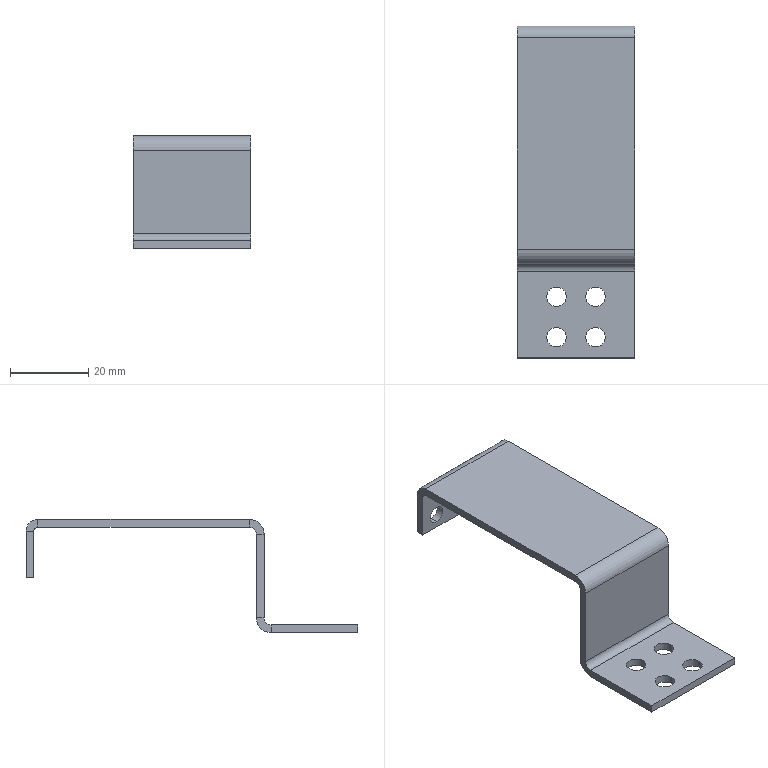Part | SolidWorks | features EdgeFlange 3, HoleWzd 2, FlatPattern 1, SMBaseFlange 1, SheetMetal 1 | 1 solid | 42 faces | box 30 x 85 x 29 mm | volume 7084 mm3 | plane 24 | cylinder 18 | commonest cylinder face diameters 5 x8 4.5 x4 3.6 x2 7.6 x2 2 x1 6 x1
STEP:
#1=CARTESIAN_POINT('',(-59.759,21.133,-13.25));
#2=VERTEX_POINT('',#1);
#3=CARTESIAN_POINT('',(-59.759,21.133,-8.75));
#4=VERTEX_POINT('',#3);
#5=CARTESIAN_POINT('',(-59.759,21.133,-11.));
#6=DIRECTION('',(0.,1.,0.));
#7=DIRECTION('',(0.,0.,1.));
#8=AXIS2_PLACEMENT_3D('',#5,#6,#7);
#9=CIRCLE('',#8,2.25);
#10=EDGE_CURVE('',#2,#4,#9,.T.);
#11=ORIENTED_EDGE('',*,*,#10,.T.);
#12=CARTESIAN_POINT('',(-59.759,19.133,-8.75));
#13=VERTEX_POINT('',#12);
#14=CARTESIAN_POINT('',(-59.759,19.133,-8.75));
#15=DIRECTION('',(0.,-1.,0.));
#16=VECTOR('',#15,1000.);
#17=LINE('',#14,#16);
#18=EDGE_CURVE('',#4,#13,#17,.T.);
#19=ORIENTED_EDGE('',*,*,#18,.T.);
#20=CARTESIAN_POINT('',(-59.759,19.133,-13.25));
#21=VERTEX_POINT('',#20);
#22=CARTESIAN_POINT('',(-59.759,19.133,-11.));
#23=DIRECTION('',(0.,-1.,0.));
#24=DIRECTION('',(0.,0.,-1.));
#25=AXIS2_PLACEMENT_3D('',#22,#23,#24);
#26=CIRCLE('',#25,2.25);
#27=EDGE_CURVE('',#13,#21,#26,.T.);
#28=ORIENTED_EDGE('',*,*,#27,.T.);
#29=CARTESIAN_POINT('',(-59.759,19.133,-13.25));
#30=DIRECTION('',(0.,-1.,0.));
#31=VECTOR('',#30,1000.);
#32=LINE('',#29,#31);
#33=EDGE_CURVE('',#2,#21,#32,.T.);
#34=ORIENTED_EDGE('',*,*,#33,.F.);
#35=EDGE_LOOP('',(#11,#19,#28,#34));
#36=FACE_OUTER_BOUND('',#35,.T.);
#37=CARTESIAN_POINT('',(-59.759,19.133,-11.));
#38=DIRECTION('',(0.,-1.,0.));
#39=DIRECTION('',(0.,0.,-1.));
#40=AXIS2_PLACEMENT_3D('',#37,#38,#39);
#41=CYLINDRICAL_SURFACE('',#40,2.25);
#42=ADVANCED_FACE('',(#36),#41,.F.);
#43=CARTESIAN_POINT('',(-39.759,21.133,-13.25));
#44=VERTEX_POINT('',#43);
#45=CARTESIAN_POINT('',(-39.759,21.133,-8.75));
#46=VERTEX_POINT('',#45);
#47=CARTESIAN_POINT('',(-39.759,21.133,-11.));
#48=DIRECTION('',(0.,1.,0.));
#49=DIRECTION('',(0.,0.,1.));
#50=AXIS2_PLACEMENT_3D('',#47,#48,#49);
#51=CIRCLE('',#50,2.25);
#52=EDGE_CURVE('',#44,#46,#51,.T.);
#53=ORIENTED_EDGE('',*,*,#52,.T.);
#54=CARTESIAN_POINT('',(-39.759,19.133,-8.75));
#55=VERTEX_POINT('',#54);
#56=CARTESIAN_POINT('',(-39.759,19.133,-8.75));
#57=DIRECTION('',(0.,-1.,0.));
#58=VECTOR('',#57,1000.);
#59=LINE('',#56,#58);
#60=EDGE_CURVE('',#46,#55,#59,.T.);
#61=ORIENTED_EDGE('',*,*,#60,.T.);
#62=CARTESIAN_POINT('',(-39.759,19.133,-13.25));
#63=VERTEX_POINT('',#62);
#64=CARTESIAN_POINT('',(-39.759,19.133,-11.));
#65=DIRECTION('',(0.,-1.,0.));
#66=DIRECTION('',(0.,0.,-1.));
#67=AXIS2_PLACEMENT_3D('',#64,#65,#66);
#68=CIRCLE('',#67,2.25);
#69=EDGE_CURVE('',#55,#63,#68,.T.);
#70=ORIENTED_EDGE('',*,*,#69,.T.);
#71=CARTESIAN_POINT('',(-39.759,19.133,-13.25));
#72=DIRECTION('',(0.,-1.,0.));
#73=VECTOR('',#72,1000.);
#74=LINE('',#71,#73);
#75=EDGE_CURVE('',#44,#63,#74,.T.);
#76=ORIENTED_EDGE('',*,*,#75,.F.);
#77=EDGE_LOOP('',(#53,#61,#70,#76));
#78=FACE_OUTER_BOUND('',#77,.T.);
#79=CARTESIAN_POINT('',(-39.759,19.133,-11.));
#80=DIRECTION('',(0.,-1.,0.));
#81=DIRECTION('',(0.,0.,-1.));
#82=AXIS2_PLACEMENT_3D('',#79,#80,#81);
#83=CYLINDRICAL_SURFACE('',#82,2.25);
#84=ADVANCED_FACE('',(#78),#83,.F.);
#85=CARTESIAN_POINT('',(-57.259,-48.167,-29.));
#86=VERTEX_POINT('',#85);
#87=CARTESIAN_POINT('',(-52.259,-48.167,-29.));
#88=VERTEX_POINT('',#87);
#89=CARTESIAN_POINT('',(-54.759,-48.167,-29.));
#90=DIRECTION('',(0.,0.,1.));
#91=DIRECTION('',(0.,-1.,0.));
#92=AXIS2_PLACEMENT_3D('',#89,#90,#91);
#93=CIRCLE('',#92,2.5);
#94=EDGE_CURVE('',#86,#88,#93,.T.);
#95=ORIENTED_EDGE('',*,*,#94,.F.);
#96=CARTESIAN_POINT('',(-57.259,-48.167,-27.));
#97=VERTEX_POINT('',#96);
#98=CARTESIAN_POINT('',(-57.259,-48.167,-27.));
#99=DIRECTION('',(0.,0.,1.));
#100=VECTOR('',#99,1000.);
#101=LINE('',#98,#100);
#102=EDGE_CURVE('',#86,#97,#101,.T.);
#103=ORIENTED_EDGE('',*,*,#102,.T.);
#104=CARTESIAN_POINT('',(-52.259,-48.167,-27.));
#105=VERTEX_POINT('',#104);
#106=CARTESIAN_POINT('',(-54.759,-48.167,-27.));
#107=DIRECTION('',(0.,0.,1.));
#108=DIRECTION('',(1.,0.,0.));
#109=AXIS2_PLACEMENT_3D('',#106,#107,#108);
#110=CIRCLE('',#109,2.5);
#111=EDGE_CURVE('',#97,#105,#110,.T.);
#112=ORIENTED_EDGE('',*,*,#111,.T.);
#113=CARTESIAN_POINT('',(-52.259,-48.167,-27.));
#114=DIRECTION('',(0.,0.,1.));
#115=VECTOR('',#114,1000.);
#116=LINE('',#113,#115);
#117=EDGE_CURVE('',#88,#105,#116,.T.);
#118=ORIENTED_EDGE('',*,*,#117,.F.);
#119=EDGE_LOOP('',(#95,#103,#112,#118));
#120=FACE_OUTER_BOUND('',#119,.T.);
#121=CARTESIAN_POINT('',(-54.759,-48.167,-27.));
#122=DIRECTION('',(0.,0.,1.));
#123=DIRECTION('',(1.,0.,0.));
#124=AXIS2_PLACEMENT_3D('',#121,#122,#123);
#125=CYLINDRICAL_SURFACE('',#124,2.5);
#126=ADVANCED_FACE('',(#120),#125,.F.);
#127=CARTESIAN_POINT('',(-47.259,-48.167,-29.));
#128=VERTEX_POINT('',#127);
#129=CARTESIAN_POINT('',(-42.259,-48.167,-29.));
#130=VERTEX_POINT('',#129);
#131=CARTESIAN_POINT('',(-44.759,-48.167,-29.));
#132=DIRECTION('',(0.,0.,1.));
#133=DIRECTION('',(0.,-1.,0.));
#134=AXIS2_PLACEMENT_3D('',#131,#132,#133);
#135=CIRCLE('',#134,2.5);
#136=EDGE_CURVE('',#128,#130,#135,.T.);
#137=ORIENTED_EDGE('',*,*,#136,.F.);
#138=CARTESIAN_POINT('',(-47.259,-48.167,-27.));
#139=VERTEX_POINT('',#138);
#140=CARTESIAN_POINT('',(-47.259,-48.167,-27.));
#141=DIRECTION('',(0.,0.,1.));
#142=VECTOR('',#141,1000.);
#143=LINE('',#140,#142);
#144=EDGE_CURVE('',#128,#139,#143,.T.);
#145=ORIENTED_EDGE('',*,*,#144,.T.);
#146=CARTESIAN_POINT('',(-42.259,-48.167,-27.));
#147=VERTEX_POINT('',#146);
#148=CARTESIAN_POINT('',(-44.759,-48.167,-27.));
#149=DIRECTION('',(0.,0.,1.));
#150=DIRECTION('',(1.,0.,0.));
#151=AXIS2_PLACEMENT_3D('',#148,#149,#150);
#152=CIRCLE('',#151,2.5);
#153=EDGE_CURVE('',#139,#147,#152,.T.);
#154=ORIENTED_EDGE('',*,*,#153,.T.);
#155=CARTESIAN_POINT('',(-42.259,-48.167,-27.));
#156=DIRECTION('',(0.,0.,1.));
#157=VECTOR('',#156,1000.);
#158=LINE('',#155,#157);
#159=EDGE_CURVE('',#130,#147,#158,.T.);
#160=ORIENTED_EDGE('',*,*,#159,.F.);
#161=EDGE_LOOP('',(#137,#145,#154,#160));
#162=FACE_OUTER_BOUND('',#161,.T.);
#163=CARTESIAN_POINT('',(-44.759,-48.167,-27.));
#164=DIRECTION('',(0.,0.,1.));
#165=DIRECTION('',(1.,0.,0.));
#166=AXIS2_PLACEMENT_3D('',#163,#164,#165);
#167=CYLINDRICAL_SURFACE('',#166,2.5);
#168=ADVANCED_FACE('',(#162),#167,.F.);
#169=CARTESIAN_POINT('',(-47.259,-58.567,-29.));
#170=VERTEX_POINT('',#169);
#171=CARTESIAN_POINT('',(-42.259,-58.567,-29.));
#172=VERTEX_POINT('',#171);
#173=CARTESIAN_POINT('',(-44.759,-58.567,-29.));
#174=DIRECTION('',(0.,0.,1.));
#175=DIRECTION('',(0.,-1.,0.));
#176=AXIS2_PLACEMENT_3D('',#173,#174,#175);
#177=CIRCLE('',#176,2.5);
#178=EDGE_CURVE('',#170,#172,#177,.T.);
#179=ORIENTED_EDGE('',*,*,#178,.F.);
#180=CARTESIAN_POINT('',(-47.259,-58.567,-27.));
#181=VERTEX_POINT('',#180);
#182=CARTESIAN_POINT('',(-47.259,-58.567,-27.));
#183=DIRECTION('',(0.,0.,1.));
#184=VECTOR('',#183,1000.);
#185=LINE('',#182,#184);
#186=EDGE_CURVE('',#170,#181,#185,.T.);
#187=ORIENTED_EDGE('',*,*,#186,.T.);
#188=CARTESIAN_POINT('',(-42.259,-58.567,-27.));
#189=VERTEX_POINT('',#188);
#190=CARTESIAN_POINT('',(-44.759,-58.567,-27.));
#191=DIRECTION('',(0.,0.,1.));
#192=DIRECTION('',(1.,0.,0.));
#193=AXIS2_PLACEMENT_3D('',#190,#191,#192);
#194=CIRCLE('',#193,2.5);
#195=EDGE_CURVE('',#181,#189,#194,.T.);
#196=ORIENTED_EDGE('',*,*,#195,.T.);
#197=CARTESIAN_POINT('',(-42.259,-58.567,-27.));
#198=DIRECTION('',(0.,0.,1.));
#199=VECTOR('',#198,1000.);
#200=LINE('',#197,#199);
#201=EDGE_CURVE('',#172,#189,#200,.T.);
#202=ORIENTED_EDGE('',*,*,#201,.F.);
#203=EDGE_LOOP('',(#179,#187,#196,#202));
#204=FACE_OUTER_BOUND('',#203,.T.);
#205=CARTESIAN_POINT('',(-44.759,-58.567,-27.));
#206=DIRECTION('',(0.,0.,1.));
#207=DIRECTION('',(1.,0.,0.));
#208=AXIS2_PLACEMENT_3D('',#205,#206,#207);
#209=CYLINDRICAL_SURFACE('',#208,2.5);
#210=ADVANCED_FACE('',(#204),#209,.F.);
#211=CARTESIAN_POINT('',(-57.259,-58.567,-29.));
#212=VERTEX_POINT('',#211);
#213=CARTESIAN_POINT('',(-52.259,-58.567,-29.));
#214=VERTEX_POINT('',#213);
#215=CARTESIAN_POINT('',(-54.759,-58.567,-29.));
#216=DIRECTION('',(0.,0.,1.));
#217=DIRECTION('',(0.,-1.,0.));
#218=AXIS2_PLACEMENT_3D('',#215,#216,#217);
#219=CIRCLE('',#218,2.5);
#220=EDGE_CURVE('',#212,#214,#219,.T.);
#221=ORIENTED_EDGE('',*,*,#220,.F.);
#222=CARTESIAN_POINT('',(-57.259,-58.567,-27.));
#223=VERTEX_POINT('',#222);
#224=CARTESIAN_POINT('',(-57.259,-58.567,-27.));
#225=DIRECTION('',(0.,0.,1.));
#226=VECTOR('',#225,1000.);
#227=LINE('',#224,#226);
#228=EDGE_CURVE('',#212,#223,#227,.T.);
#229=ORIENTED_EDGE('',*,*,#228,.T.);
#230=CARTESIAN_POINT('',(-52.259,-58.567,-27.));
#231=VERTEX_POINT('',#230);
#232=CARTESIAN_POINT('',(-54.759,-58.567,-27.));
#233=DIRECTION('',(0.,0.,1.));
#234=DIRECTION('',(1.,0.,0.));
#235=AXIS2_PLACEMENT_3D('',#232,#233,#234);
#236=CIRCLE('',#235,2.5);
#237=EDGE_CURVE('',#223,#231,#236,.T.);
#238=ORIENTED_EDGE('',*,*,#237,.T.);
#239=CARTESIAN_POINT('',(-52.259,-58.567,-27.));
#240=DIRECTION('',(0.,0.,1.));
#241=VECTOR('',#240,1000.);
#242=LINE('',#239,#241);
#243=EDGE_CURVE('',#214,#231,#242,.T.);
#244=ORIENTED_EDGE('',*,*,#243,.F.);
#245=EDGE_LOOP('',(#221,#229,#238,#244));
#246=FACE_OUTER_BOUND('',#245,.T.);
#247=CARTESIAN_POINT('',(-54.759,-58.567,-27.));
#248=DIRECTION('',(0.,0.,1.));
#249=DIRECTION('',(1.,0.,0.));
#250=AXIS2_PLACEMENT_3D('',#247,#248,#249);
#251=CYLINDRICAL_SURFACE('',#250,2.5);
#252=ADVANCED_FACE('',(#246),#251,.F.);
#253=CARTESIAN_POINT('',(-34.759,18.133,-2.));
#254=VERTEX_POINT('',#253);
#255=CARTESIAN_POINT('',(-64.759,18.133,-2.));
#256=VERTEX_POINT('',#255);
#257=CARTESIAN_POINT('',(-34.759,18.133,-2.));
#258=DIRECTION('',(-1.,0.,0.));
#259=VECTOR('',#258,1000.);
#260=LINE('',#257,#259);
#261=EDGE_CURVE('',#254,#256,#260,.T.);
#262=ORIENTED_EDGE('',*,*,#261,.F.);
#263=CARTESIAN_POINT('',(-34.759,-36.067,-2.));
#264=VERTEX_POINT('',#263);
#265=CARTESIAN_POINT('',(-34.759,19.133,-2.));
#266=DIRECTION('',(0.,1.,0.));
#267=VECTOR('',#266,1000.);
#268=LINE('',#265,#267);
#269=EDGE_CURVE('',#264,#254,#268,.T.);
#270=ORIENTED_EDGE('',*,*,#269,.F.);
#271=CARTESIAN_POINT('',(-64.759,-36.067,-2.));
#272=VERTEX_POINT('',#271);
#273=CARTESIAN_POINT('',(-64.759,-36.067,-2.));
#274=DIRECTION('',(1.,0.,0.));
#275=VECTOR('',#274,1000.);
#276=LINE('',#273,#275);
#277=EDGE_CURVE('',#272,#264,#276,.T.);
#278=ORIENTED_EDGE('',*,*,#277,.F.);
#279=CARTESIAN_POINT('',(-64.759,19.133,-2.));
#280=DIRECTION('',(0.,-1.,0.));
#281=VECTOR('',#280,1000.);
#282=LINE('',#279,#281);
#283=EDGE_CURVE('',#256,#272,#282,.T.);
#284=ORIENTED_EDGE('',*,*,#283,.F.);
#285=EDGE_LOOP('',(#262,#270,#278,#284));
#286=FACE_OUTER_BOUND('',#285,.T.);
#287=CARTESIAN_POINT('',(0.,0.,-2.));
#288=DIRECTION('',(0.,0.,1.));
#289=DIRECTION('',(1.,0.,0.));
#290=AXIS2_PLACEMENT_3D('',#287,#288,#289);
#291=PLANE('',#290);
#292=ADVANCED_FACE('',(#286),#291,.F.);
#293=CARTESIAN_POINT('',(-34.759,-36.067,0.));
#294=VERTEX_POINT('',#293);
#295=CARTESIAN_POINT('',(-34.759,18.133,0.));
#296=VERTEX_POINT('',#295);
#297=CARTESIAN_POINT('',(-34.759,19.133,0.));
#298=DIRECTION('',(0.,1.,0.));
#299=VECTOR('',#298,1000.);
#300=LINE('',#297,#299);
#301=EDGE_CURVE('',#294,#296,#300,.T.);
#302=ORIENTED_EDGE('',*,*,#301,.T.);
#303=CARTESIAN_POINT('',(-64.759,18.133,0.));
#304=VERTEX_POINT('',#303);
#305=CARTESIAN_POINT('',(-34.759,18.133,0.));
#306=DIRECTION('',(-1.,0.,0.));
#307=VECTOR('',#306,1000.);
#308=LINE('',#305,#307);
#309=EDGE_CURVE('',#296,#304,#308,.T.);
#310=ORIENTED_EDGE('',*,*,#309,.T.);
#311=CARTESIAN_POINT('',(-64.759,-36.067,0.));
#312=VERTEX_POINT('',#311);
#313=CARTESIAN_POINT('',(-64.759,19.133,0.));
#314=DIRECTION('',(0.,-1.,0.));
#315=VECTOR('',#314,1000.);
#316=LINE('',#313,#315);
#317=EDGE_CURVE('',#304,#312,#316,.T.);
#318=ORIENTED_EDGE('',*,*,#317,.T.);
#319=CARTESIAN_POINT('',(-64.759,-36.067,0.));
#320=DIRECTION('',(1.,0.,0.));
#321=VECTOR('',#320,1000.);
#322=LINE('',#319,#321);
#323=EDGE_CURVE('',#312,#294,#322,.T.);
#324=ORIENTED_EDGE('',*,*,#323,.T.);
#325=EDGE_LOOP('',(#302,#310,#318,#324));
#326=FACE_OUTER_BOUND('',#325,.T.);
#327=CARTESIAN_POINT('',(0.,0.,0.));
#328=DIRECTION('',(0.,0.,1.));
#329=DIRECTION('',(1.,0.,0.));
#330=AXIS2_PLACEMENT_3D('',#327,#328,#329);
#331=PLANE('',#330);
#332=ADVANCED_FACE('',(#326),#331,.T.);
#333=ORIENTED_EDGE('',*,*,#269,.T.);
#334=CARTESIAN_POINT('',(-34.759,18.133,-2.));
#335=DIRECTION('',(0.,0.,1.));
#336=VECTOR('',#335,1000.);
#337=LINE('',#334,#336);
#338=EDGE_CURVE('',#254,#296,#337,.T.);
#339=ORIENTED_EDGE('',*,*,#338,.T.);
#340=ORIENTED_EDGE('',*,*,#301,.F.);
#341=CARTESIAN_POINT('',(-34.759,-36.067,-2.));
#342=DIRECTION('',(0.,0.,1.));
#343=VECTOR('',#342,1000.);
#344=LINE('',#341,#343);
#345=EDGE_CURVE('',#264,#294,#344,.T.);
#346=ORIENTED_EDGE('',*,*,#345,.F.);
#347=EDGE_LOOP('',(#333,#339,#340,#346));
#348=FACE_OUTER_BOUND('',#347,.T.);
#349=CARTESIAN_POINT('',(-34.759,19.133,-2.));
#350=DIRECTION('',(1.,0.,0.));
#351=DIRECTION('',(0.,1.,0.));
#352=AXIS2_PLACEMENT_3D('',#349,#350,#351);
#353=PLANE('',#352);
#354=ADVANCED_FACE('',(#348),#353,.T.);
#355=CARTESIAN_POINT('',(-64.759,-39.867,-25.2));
#356=VERTEX_POINT('',#355);
#357=CARTESIAN_POINT('',(-64.759,-37.867,-25.2));
#358=VERTEX_POINT('',#357);
#359=CARTESIAN_POINT('',(-64.759,-39.867,-25.2));
#360=DIRECTION('',(0.,1.,0.));
#361=VECTOR('',#360,1000.);
#362=LINE('',#359,#361);
#363=EDGE_CURVE('',#356,#358,#362,.T.);
#364=ORIENTED_EDGE('',*,*,#363,.F.);
#365=CARTESIAN_POINT('',(-64.759,-39.867,-3.8));
#366=VERTEX_POINT('',#365);
#367=CARTESIAN_POINT('',(-64.759,-39.867,-27.));
#368=DIRECTION('',(0.,0.,-1.));
#369=VECTOR('',#368,1000.);
#370=LINE('',#367,#369);
#371=EDGE_CURVE('',#366,#356,#370,.T.);
#372=ORIENTED_EDGE('',*,*,#371,.F.);
#373=CARTESIAN_POINT('',(-64.759,-37.867,-3.8));
#374=VERTEX_POINT('',#373);
#375=CARTESIAN_POINT('',(-64.759,-37.867,-3.8));
#376=DIRECTION('',(0.,-1.,0.));
#377=VECTOR('',#376,1000.);
#378=LINE('',#375,#377);
#379=EDGE_CURVE('',#374,#366,#378,.T.);
#380=ORIENTED_EDGE('',*,*,#379,.F.);
#381=CARTESIAN_POINT('',(-64.759,-37.867,-27.));
#382=DIRECTION('',(0.,0.,-1.));
#383=VECTOR('',#382,1000.);
#384=LINE('',#381,#383);
#385=EDGE_CURVE('',#374,#358,#384,.T.);
#386=ORIENTED_EDGE('',*,*,#385,.T.);
#387=EDGE_LOOP('',(#364,#372,#380,#386));
#388=FACE_OUTER_BOUND('',#387,.T.);
#389=CARTESIAN_POINT('',(-64.759,-39.867,-27.));
#390=DIRECTION('',(1.,0.,0.));
#391=DIRECTION('',(0.,0.,-1.));
#392=AXIS2_PLACEMENT_3D('',#389,#390,#391);
#393=PLANE('',#392);
#394=ADVANCED_FACE('',(#388),#393,.F.);
#395=CARTESIAN_POINT('',(-34.759,-39.867,-25.2));
#396=VERTEX_POINT('',#395);
#397=CARTESIAN_POINT('',(-34.759,-37.867,-25.2));
#398=VERTEX_POINT('',#397);
#399=CARTESIAN_POINT('',(-34.759,-39.867,-25.2));
#400=DIRECTION('',(0.,1.,0.));
#401=VECTOR('',#400,1000.);
#402=LINE('',#399,#401);
#403=EDGE_CURVE('',#396,#398,#402,.T.);
#404=ORIENTED_EDGE('',*,*,#403,.T.);
#405=CARTESIAN_POINT('',(-34.759,-37.867,-3.8));
#406=VERTEX_POINT('',#405);
#407=CARTESIAN_POINT('',(-34.759,-37.867,-2.));
#408=DIRECTION('',(0.,0.,1.));
#409=VECTOR('',#408,1000.);
#410=LINE('',#407,#409);
#411=EDGE_CURVE('',#398,#406,#410,.T.);
#412=ORIENTED_EDGE('',*,*,#411,.T.);
#413=CARTESIAN_POINT('',(-34.759,-39.867,-3.8));
#414=VERTEX_POINT('',#413);
#415=CARTESIAN_POINT('',(-34.759,-37.867,-3.8));
#416=DIRECTION('',(0.,-1.,0.));
#417=VECTOR('',#416,1000.);
#418=LINE('',#415,#417);
#419=EDGE_CURVE('',#406,#414,#418,.T.);
#420=ORIENTED_EDGE('',*,*,#419,.T.);
#421=CARTESIAN_POINT('',(-34.759,-39.867,-2.));
#422=DIRECTION('',(0.,0.,1.));
#423=VECTOR('',#422,1000.);
#424=LINE('',#421,#423);
#425=EDGE_CURVE('',#396,#414,#424,.T.);
#426=ORIENTED_EDGE('',*,*,#425,.F.);
#427=EDGE_LOOP('',(#404,#412,#420,#426));
#428=FACE_OUTER_BOUND('',#427,.T.);
#429=CARTESIAN_POINT('',(-34.759,-39.867,-2.));
#430=DIRECTION('',(-1.,0.,0.));
#431=DIRECTION('',(0.,0.,1.));
#432=AXIS2_PLACEMENT_3D('',#429,#430,#431);
#433=PLANE('',#432);
#434=ADVANCED_FACE('',(#428),#433,.F.);
#435=CARTESIAN_POINT('',(-34.759,-39.867,-25.2));
#436=DIRECTION('',(-1.,0.,0.));
#437=VECTOR('',#436,1000.);
#438=LINE('',#435,#437);
#439=EDGE_CURVE('',#396,#356,#438,.T.);
#440=ORIENTED_EDGE('',*,*,#439,.F.);
#441=ORIENTED_EDGE('',*,*,#425,.T.);
#442=CARTESIAN_POINT('',(0.,-39.867,-3.8));
#443=DIRECTION('',(1.,0.,0.));
#444=VECTOR('',#443,1000.);
#445=LINE('',#442,#444);
#446=EDGE_CURVE('',#366,#414,#445,.T.);
#447=ORIENTED_EDGE('',*,*,#446,.F.);
#448=ORIENTED_EDGE('',*,*,#371,.T.);
#449=EDGE_LOOP('',(#440,#441,#447,#448));
#450=FACE_OUTER_BOUND('',#449,.T.);
#451=CARTESIAN_POINT('',(0.,-39.867,0.));
#452=DIRECTION('',(0.,1.,0.));
#453=DIRECTION('',(0.,0.,1.));
#454=AXIS2_PLACEMENT_3D('',#451,#452,#453);
#455=PLANE('',#454);
#456=ADVANCED_FACE('',(#450),#455,.F.);
#457=ORIENTED_EDGE('',*,*,#411,.F.);
#458=CARTESIAN_POINT('',(-34.759,-37.867,-25.2));
#459=DIRECTION('',(-1.,0.,0.));
#460=VECTOR('',#459,1000.);
#461=LINE('',#458,#460);
#462=EDGE_CURVE('',#398,#358,#461,.T.);
#463=ORIENTED_EDGE('',*,*,#462,.T.);
#464=ORIENTED_EDGE('',*,*,#385,.F.);
#465=CARTESIAN_POINT('',(-34.759,-37.867,-3.8));
#466=DIRECTION('',(-1.,0.,0.));
#467=VECTOR('',#466,1000.);
#468=LINE('',#465,#467);
#469=EDGE_CURVE('',#406,#374,#468,.T.);
#470=ORIENTED_EDGE('',*,*,#469,.F.);
#471=EDGE_LOOP('',(#457,#463,#464,#470));
#472=FACE_OUTER_BOUND('',#471,.T.);
#473=CARTESIAN_POINT('',(0.,-37.867,0.));
#474=DIRECTION('',(0.,1.,0.));
#475=DIRECTION('',(0.,0.,1.));
#476=AXIS2_PLACEMENT_3D('',#473,#474,#475);
#477=PLANE('',#476);
#478=ADVANCED_FACE('',(#472),#477,.T.);
#479=CARTESIAN_POINT('',(-64.759,18.133,-2.));
#480=DIRECTION('',(0.,0.,1.));
#481=VECTOR('',#480,1000.);
#482=LINE('',#479,#481);
#483=EDGE_CURVE('',#256,#304,#482,.T.);
#484=ORIENTED_EDGE('',*,*,#483,.F.);
#485=ORIENTED_EDGE('',*,*,#283,.T.);
#486=CARTESIAN_POINT('',(-64.759,-36.067,-2.));
#487=DIRECTION('',(0.,0.,1.));
#488=VECTOR('',#487,1000.);
#489=LINE('',#486,#488);
#490=EDGE_CURVE('',#272,#312,#489,.T.);
#491=ORIENTED_EDGE('',*,*,#490,.T.);
#492=ORIENTED_EDGE('',*,*,#317,.F.);
#493=EDGE_LOOP('',(#484,#485,#491,#492));
#494=FACE_OUTER_BOUND('',#493,.T.);
#495=CARTESIAN_POINT('',(-64.759,19.133,-2.));
#496=DIRECTION('',(-1.,0.,0.));
#497=DIRECTION('',(0.,-1.,0.));
#498=AXIS2_PLACEMENT_3D('',#495,#496,#497);
#499=PLANE('',#498);
#500=ADVANCED_FACE('',(#494),#499,.T.);
#501=ORIENTED_EDGE('',*,*,#419,.F.);
#502=CARTESIAN_POINT('',(-34.759,-36.067,-3.8));
#503=DIRECTION('',(1.,0.,0.));
#504=DIRECTION('',(0.,0.,1.));
#505=AXIS2_PLACEMENT_3D('',#502,#503,#504);
#506=CIRCLE('',#505,1.8);
#507=EDGE_CURVE('',#264,#406,#506,.T.);
#508=ORIENTED_EDGE('',*,*,#507,.F.);
#509=ORIENTED_EDGE('',*,*,#345,.T.);
#510=CARTESIAN_POINT('',(-34.759,-36.067,-3.8));
#511=DIRECTION('',(1.,0.,0.));
#512=DIRECTION('',(0.,0.,1.));
#513=AXIS2_PLACEMENT_3D('',#510,#511,#512);
#514=CIRCLE('',#513,3.8);
#515=EDGE_CURVE('',#294,#414,#514,.T.);
#516=ORIENTED_EDGE('',*,*,#515,.T.);
#517=EDGE_LOOP('',(#501,#508,#509,#516));
#518=FACE_OUTER_BOUND('',#517,.T.);
#519=CARTESIAN_POINT('',(-34.759,-36.067,-3.8));
#520=DIRECTION('',(1.,0.,0.));
#521=DIRECTION('',(0.,0.,-1.));
#522=AXIS2_PLACEMENT_3D('',#519,#520,#521);
#523=PLANE('',#522);
#524=ADVANCED_FACE('',(#518),#523,.T.);
#525=CARTESIAN_POINT('',(-64.759,-36.067,-3.8));
#526=DIRECTION('',(-1.,0.,0.));
#527=DIRECTION('',(0.,0.,1.));
#528=AXIS2_PLACEMENT_3D('',#525,#526,#527);
#529=CIRCLE('',#528,1.8);
#530=EDGE_CURVE('',#374,#272,#529,.T.);
#531=ORIENTED_EDGE('',*,*,#530,.F.);
#532=ORIENTED_EDGE('',*,*,#379,.T.);
#533=CARTESIAN_POINT('',(-64.759,-36.067,-3.8));
#534=DIRECTION('',(-1.,0.,0.));
#535=DIRECTION('',(0.,0.,1.));
#536=AXIS2_PLACEMENT_3D('',#533,#534,#535);
#537=CIRCLE('',#536,3.8);
#538=EDGE_CURVE('',#366,#312,#537,.T.);
#539=ORIENTED_EDGE('',*,*,#538,.T.);
#540=ORIENTED_EDGE('',*,*,#490,.F.);
#541=EDGE_LOOP('',(#531,#532,#539,#540));
#542=FACE_OUTER_BOUND('',#541,.T.);
#543=CARTESIAN_POINT('',(-64.759,-36.067,-3.8));
#544=DIRECTION('',(1.,0.,0.));
#545=DIRECTION('',(0.,0.,-1.));
#546=AXIS2_PLACEMENT_3D('',#543,#544,#545);
#547=PLANE('',#546);
#548=ADVANCED_FACE('',(#542),#547,.F.);
#549=ORIENTED_EDGE('',*,*,#323,.F.);
#550=ORIENTED_EDGE('',*,*,#538,.F.);
#551=ORIENTED_EDGE('',*,*,#446,.T.);
#552=ORIENTED_EDGE('',*,*,#515,.F.);
#553=EDGE_LOOP('',(#549,#550,#551,#552));
#554=FACE_OUTER_BOUND('',#553,.T.);
#555=CARTESIAN_POINT('',(-64.759,-36.067,-3.8));
#556=DIRECTION('',(-1.,0.,0.));
#557=DIRECTION('',(0.,-1.,0.));
#558=AXIS2_PLACEMENT_3D('',#555,#556,#557);
#559=CYLINDRICAL_SURFACE('',#558,3.8);
#560=ADVANCED_FACE('',(#554),#559,.T.);
#561=ORIENTED_EDGE('',*,*,#277,.T.);
#562=ORIENTED_EDGE('',*,*,#507,.T.);
#563=ORIENTED_EDGE('',*,*,#469,.T.);
#564=ORIENTED_EDGE('',*,*,#530,.T.);
#565=EDGE_LOOP('',(#561,#562,#563,#564));
#566=FACE_OUTER_BOUND('',#565,.T.);
#567=CARTESIAN_POINT('',(-64.759,-36.067,-3.8));
#568=DIRECTION('',(-1.,0.,0.));
#569=DIRECTION('',(0.,-1.,0.));
#570=AXIS2_PLACEMENT_3D('',#567,#568,#569);
#571=CYLINDRICAL_SURFACE('',#570,1.8);
#572=ADVANCED_FACE('',(#566),#571,.F.);
#573=CARTESIAN_POINT('',(-64.759,-41.667,-27.));
#574=VERTEX_POINT('',#573);
#575=CARTESIAN_POINT('',(-64.759,-41.667,-29.));
#576=VERTEX_POINT('',#575);
#577=CARTESIAN_POINT('',(-64.759,-41.667,-27.));
#578=DIRECTION('',(0.,0.,-1.));
#579=VECTOR('',#578,1000.);
#580=LINE('',#577,#579);
#581=EDGE_CURVE('',#574,#576,#580,.T.);
#582=ORIENTED_EDGE('',*,*,#581,.F.);
#583=CARTESIAN_POINT('',(-64.759,-41.667,-25.2));
#584=DIRECTION('',(-1.,0.,0.));
#585=DIRECTION('',(0.,0.,-1.));
#586=AXIS2_PLACEMENT_3D('',#583,#584,#585);
#587=CIRCLE('',#586,1.8);
#588=EDGE_CURVE('',#356,#574,#587,.T.);
#589=ORIENTED_EDGE('',*,*,#588,.F.);
#590=ORIENTED_EDGE('',*,*,#363,.T.);
#591=CARTESIAN_POINT('',(-64.759,-41.667,-25.2));
#592=DIRECTION('',(-1.,0.,0.));
#593=DIRECTION('',(0.,0.,-1.));
#594=AXIS2_PLACEMENT_3D('',#591,#592,#593);
#595=CIRCLE('',#594,3.8);
#596=EDGE_CURVE('',#358,#576,#595,.T.);
#597=ORIENTED_EDGE('',*,*,#596,.T.);
#598=EDGE_LOOP('',(#582,#589,#590,#597));
#599=FACE_OUTER_BOUND('',#598,.T.);
#600=CARTESIAN_POINT('',(-64.759,-41.667,-25.2));
#601=DIRECTION('',(-1.,0.,0.));
#602=DIRECTION('',(0.,0.,1.));
#603=AXIS2_PLACEMENT_3D('',#600,#601,#602);
#604=PLANE('',#603);
#605=ADVANCED_FACE('',(#599),#604,.T.);
#606=CARTESIAN_POINT('',(-34.759,-41.667,-27.));
#607=VERTEX_POINT('',#606);
#608=CARTESIAN_POINT('',(-34.759,-41.667,-25.2));
#609=DIRECTION('',(1.,0.,0.));
#610=DIRECTION('',(0.,0.,-1.));
#611=AXIS2_PLACEMENT_3D('',#608,#609,#610);
#612=CIRCLE('',#611,1.8);
#613=EDGE_CURVE('',#607,#396,#612,.T.);
#614=ORIENTED_EDGE('',*,*,#613,.F.);
#615=CARTESIAN_POINT('',(-34.759,-41.667,-29.));
#616=VERTEX_POINT('',#615);
#617=CARTESIAN_POINT('',(-34.759,-41.667,-27.));
#618=DIRECTION('',(0.,0.,-1.));
#619=VECTOR('',#618,1000.);
#620=LINE('',#617,#619);
#621=EDGE_CURVE('',#607,#616,#620,.T.);
#622=ORIENTED_EDGE('',*,*,#621,.T.);
#623=CARTESIAN_POINT('',(-34.759,-41.667,-25.2));
#624=DIRECTION('',(1.,0.,0.));
#625=DIRECTION('',(0.,0.,-1.));
#626=AXIS2_PLACEMENT_3D('',#623,#624,#625);
#627=CIRCLE('',#626,3.8);
#628=EDGE_CURVE('',#616,#398,#627,.T.);
#629=ORIENTED_EDGE('',*,*,#628,.T.);
#630=ORIENTED_EDGE('',*,*,#403,.F.);
#631=EDGE_LOOP('',(#614,#622,#629,#630));
#632=FACE_OUTER_BOUND('',#631,.T.);
#633=CARTESIAN_POINT('',(-34.759,-41.667,-25.2));
#634=DIRECTION('',(-1.,0.,0.));
#635=DIRECTION('',(0.,0.,1.));
#636=AXIS2_PLACEMENT_3D('',#633,#634,#635);
#637=PLANE('',#636);
#638=ADVANCED_FACE('',(#632),#637,.F.);
#639=ORIENTED_EDGE('',*,*,#462,.F.);
#640=ORIENTED_EDGE('',*,*,#628,.F.);
#641=CARTESIAN_POINT('',(0.,-41.667,-29.));
#642=DIRECTION('',(-1.,0.,0.));
#643=VECTOR('',#642,1000.);
#644=LINE('',#641,#643);
#645=EDGE_CURVE('',#616,#576,#644,.T.);
#646=ORIENTED_EDGE('',*,*,#645,.T.);
#647=ORIENTED_EDGE('',*,*,#596,.F.);
#648=EDGE_LOOP('',(#639,#640,#646,#647));
#649=FACE_OUTER_BOUND('',#648,.T.);
#650=CARTESIAN_POINT('',(-34.759,-41.667,-25.2));
#651=DIRECTION('',(1.,0.,0.));
#652=DIRECTION('',(0.,0.,-1.));
#653=AXIS2_PLACEMENT_3D('',#650,#651,#652);
#654=CYLINDRICAL_SURFACE('',#653,3.8);
#655=ADVANCED_FACE('',(#649),#654,.T.);
#656=ORIENTED_EDGE('',*,*,#439,.T.);
#657=ORIENTED_EDGE('',*,*,#588,.T.);
#658=CARTESIAN_POINT('',(-64.759,-41.667,-27.));
#659=DIRECTION('',(1.,0.,0.));
#660=VECTOR('',#659,1000.);
#661=LINE('',#658,#660);
#662=EDGE_CURVE('',#574,#607,#661,.T.);
#663=ORIENTED_EDGE('',*,*,#662,.T.);
#664=ORIENTED_EDGE('',*,*,#613,.T.);
#665=EDGE_LOOP('',(#656,#657,#663,#664));
#666=FACE_OUTER_BOUND('',#665,.T.);
#667=CARTESIAN_POINT('',(-34.759,-41.667,-25.2));
#668=DIRECTION('',(1.,0.,0.));
#669=DIRECTION('',(0.,0.,-1.));
#670=AXIS2_PLACEMENT_3D('',#667,#668,#669);
#671=CYLINDRICAL_SURFACE('',#670,1.8);
#672=ADVANCED_FACE('',(#666),#671,.F.);
#673=ORIENTED_EDGE('',*,*,#581,.T.);
#674=CARTESIAN_POINT('',(-64.759,-63.867,-29.));
#675=VERTEX_POINT('',#674);
#676=CARTESIAN_POINT('',(-64.759,-39.867,-29.));
#677=DIRECTION('',(0.,1.,0.));
#678=VECTOR('',#677,1000.);
#679=LINE('',#676,#678);
#680=EDGE_CURVE('',#675,#576,#679,.T.);
#681=ORIENTED_EDGE('',*,*,#680,.F.);
#682=CARTESIAN_POINT('',(-64.759,-63.867,-27.));
#683=VERTEX_POINT('',#682);
#684=CARTESIAN_POINT('',(-64.759,-63.867,-29.));
#685=DIRECTION('',(0.,0.,1.));
#686=VECTOR('',#685,1000.);
#687=LINE('',#684,#686);
#688=EDGE_CURVE('',#675,#683,#687,.T.);
#689=ORIENTED_EDGE('',*,*,#688,.T.);
#690=CARTESIAN_POINT('',(-64.759,-39.867,-27.));
#691=DIRECTION('',(0.,1.,0.));
#692=VECTOR('',#691,1000.);
#693=LINE('',#690,#692);
#694=EDGE_CURVE('',#683,#574,#693,.T.);
#695=ORIENTED_EDGE('',*,*,#694,.T.);
#696=EDGE_LOOP('',(#673,#681,#689,#695));
#697=FACE_OUTER_BOUND('',#696,.T.);
#698=CARTESIAN_POINT('',(-64.759,-39.867,-29.));
#699=DIRECTION('',(1.,0.,0.));
#700=DIRECTION('',(0.,0.,-1.));
#701=AXIS2_PLACEMENT_3D('',#698,#699,#700);
#702=PLANE('',#701);
#703=ADVANCED_FACE('',(#697),#702,.F.);
#704=ORIENTED_EDGE('',*,*,#621,.F.);
#705=CARTESIAN_POINT('',(-34.759,-63.867,-27.));
#706=VERTEX_POINT('',#705);
#707=CARTESIAN_POINT('',(-34.759,-63.867,-27.));
#708=DIRECTION('',(0.,-1.,0.));
#709=VECTOR('',#708,1000.);
#710=LINE('',#707,#709);
#711=EDGE_CURVE('',#607,#706,#710,.T.);
#712=ORIENTED_EDGE('',*,*,#711,.T.);
#713=CARTESIAN_POINT('',(-34.759,-63.867,-29.));
#714=VERTEX_POINT('',#713);
#715=CARTESIAN_POINT('',(-34.759,-63.867,-29.));
#716=DIRECTION('',(0.,0.,1.));
#717=VECTOR('',#716,1000.);
#718=LINE('',#715,#717);
#719=EDGE_CURVE('',#714,#706,#718,.T.);
#720=ORIENTED_EDGE('',*,*,#719,.F.);
#721=CARTESIAN_POINT('',(-34.759,-63.867,-29.));
#722=DIRECTION('',(0.,-1.,0.));
#723=VECTOR('',#722,1000.);
#724=LINE('',#721,#723);
#725=EDGE_CURVE('',#616,#714,#724,.T.);
#726=ORIENTED_EDGE('',*,*,#725,.F.);
#727=EDGE_LOOP('',(#704,#712,#720,#726));
#728=FACE_OUTER_BOUND('',#727,.T.);
#729=CARTESIAN_POINT('',(-34.759,-63.867,-29.));
#730=DIRECTION('',(-1.,0.,0.));
#731=DIRECTION('',(0.,0.,1.));
#732=AXIS2_PLACEMENT_3D('',#729,#730,#731);
#733=PLANE('',#732);
#734=ADVANCED_FACE('',(#728),#733,.F.);
#735=CARTESIAN_POINT('',(-54.759,-48.167,-29.));
#736=DIRECTION('',(0.,0.,1.));
#737=DIRECTION('',(0.,-1.,0.));
#738=AXIS2_PLACEMENT_3D('',#735,#736,#737);
#739=CIRCLE('',#738,2.5);
#740=EDGE_CURVE('',#88,#86,#739,.T.);
#741=ORIENTED_EDGE('',*,*,#740,.T.);
#742=ORIENTED_EDGE('',*,*,#94,.T.);
#743=EDGE_LOOP('',(#741,#742));
#744=FACE_BOUND('',#743,.T.);
#745=CARTESIAN_POINT('',(-44.759,-48.167,-29.));
#746=DIRECTION('',(0.,0.,1.));
#747=DIRECTION('',(0.,-1.,0.));
#748=AXIS2_PLACEMENT_3D('',#745,#746,#747);
#749=CIRCLE('',#748,2.5);
#750=EDGE_CURVE('',#130,#128,#749,.T.);
#751=ORIENTED_EDGE('',*,*,#750,.T.);
#752=ORIENTED_EDGE('',*,*,#136,.T.);
#753=EDGE_LOOP('',(#751,#752));
#754=FACE_BOUND('',#753,.T.);
#755=CARTESIAN_POINT('',(-44.759,-58.567,-29.));
#756=DIRECTION('',(0.,0.,1.));
#757=DIRECTION('',(0.,-1.,0.));
#758=AXIS2_PLACEMENT_3D('',#755,#756,#757);
#759=CIRCLE('',#758,2.5);
#760=EDGE_CURVE('',#172,#170,#759,.T.);
#761=ORIENTED_EDGE('',*,*,#760,.T.);
#762=ORIENTED_EDGE('',*,*,#178,.T.);
#763=EDGE_LOOP('',(#761,#762));
#764=FACE_BOUND('',#763,.T.);
#765=CARTESIAN_POINT('',(-54.759,-58.567,-29.));
#766=DIRECTION('',(0.,0.,1.));
#767=DIRECTION('',(0.,-1.,0.));
#768=AXIS2_PLACEMENT_3D('',#765,#766,#767);
#769=CIRCLE('',#768,2.5);
#770=EDGE_CURVE('',#214,#212,#769,.T.);
#771=ORIENTED_EDGE('',*,*,#770,.T.);
#772=ORIENTED_EDGE('',*,*,#220,.T.);
#773=EDGE_LOOP('',(#771,#772));
#774=FACE_BOUND('',#773,.T.);
#775=ORIENTED_EDGE('',*,*,#645,.F.);
#776=ORIENTED_EDGE('',*,*,#725,.T.);
#777=CARTESIAN_POINT('',(-64.759,-63.867,-29.));
#778=DIRECTION('',(-1.,0.,0.));
#779=VECTOR('',#778,1000.);
#780=LINE('',#777,#779);
#781=EDGE_CURVE('',#714,#675,#780,.T.);
#782=ORIENTED_EDGE('',*,*,#781,.T.);
#783=ORIENTED_EDGE('',*,*,#680,.T.);
#784=EDGE_LOOP('',(#775,#776,#782,#783));
#785=FACE_OUTER_BOUND('',#784,.T.);
#786=CARTESIAN_POINT('',(0.,0.,-29.));
#787=DIRECTION('',(0.,0.,1.));
#788=DIRECTION('',(0.,-1.,0.));
#789=AXIS2_PLACEMENT_3D('',#786,#787,#788);
#790=PLANE('',#789);
#791=ADVANCED_FACE('',(#744,#754,#764,#774,#785),#790,.F.);
#792=CARTESIAN_POINT('',(-54.759,-48.167,-27.));
#793=DIRECTION('',(0.,0.,1.));
#794=DIRECTION('',(1.,0.,0.));
#795=AXIS2_PLACEMENT_3D('',#792,#793,#794);
#796=CIRCLE('',#795,2.5);
#797=EDGE_CURVE('',#105,#97,#796,.T.);
#798=ORIENTED_EDGE('',*,*,#797,.F.);
#799=ORIENTED_EDGE('',*,*,#111,.F.);
#800=EDGE_LOOP('',(#798,#799));
#801=FACE_BOUND('',#800,.T.);
#802=CARTESIAN_POINT('',(-44.759,-48.167,-27.));
#803=DIRECTION('',(0.,0.,1.));
#804=DIRECTION('',(1.,0.,0.));
#805=AXIS2_PLACEMENT_3D('',#802,#803,#804);
#806=CIRCLE('',#805,2.5);
#807=EDGE_CURVE('',#147,#139,#806,.T.);
#808=ORIENTED_EDGE('',*,*,#807,.F.);
#809=ORIENTED_EDGE('',*,*,#153,.F.);
#810=EDGE_LOOP('',(#808,#809));
#811=FACE_BOUND('',#810,.T.);
#812=CARTESIAN_POINT('',(-44.759,-58.567,-27.));
#813=DIRECTION('',(0.,0.,1.));
#814=DIRECTION('',(1.,0.,0.));
#815=AXIS2_PLACEMENT_3D('',#812,#813,#814);
#816=CIRCLE('',#815,2.5);
#817=EDGE_CURVE('',#189,#181,#816,.T.);
#818=ORIENTED_EDGE('',*,*,#817,.F.);
#819=ORIENTED_EDGE('',*,*,#195,.F.);
#820=EDGE_LOOP('',(#818,#819));
#821=FACE_BOUND('',#820,.T.);
#822=CARTESIAN_POINT('',(-54.759,-58.567,-27.));
#823=DIRECTION('',(0.,0.,1.));
#824=DIRECTION('',(1.,0.,0.));
#825=AXIS2_PLACEMENT_3D('',#822,#823,#824);
#826=CIRCLE('',#825,2.5);
#827=EDGE_CURVE('',#231,#223,#826,.T.);
#828=ORIENTED_EDGE('',*,*,#827,.F.);
#829=ORIENTED_EDGE('',*,*,#237,.F.);
#830=EDGE_LOOP('',(#828,#829));
#831=FACE_BOUND('',#830,.T.);
#832=ORIENTED_EDGE('',*,*,#711,.F.);
#833=ORIENTED_EDGE('',*,*,#662,.F.);
#834=ORIENTED_EDGE('',*,*,#694,.F.);
#835=CARTESIAN_POINT('',(-64.759,-63.867,-27.));
#836=DIRECTION('',(-1.,0.,0.));
#837=VECTOR('',#836,1000.);
#838=LINE('',#835,#837);
#839=EDGE_CURVE('',#706,#683,#838,.T.);
#840=ORIENTED_EDGE('',*,*,#839,.F.);
#841=EDGE_LOOP('',(#832,#833,#834,#840));
#842=FACE_OUTER_BOUND('',#841,.T.);
#843=CARTESIAN_POINT('',(0.,0.,-27.));
#844=DIRECTION('',(0.,0.,1.));
#845=DIRECTION('',(0.,-1.,0.));
#846=AXIS2_PLACEMENT_3D('',#843,#844,#845);
#847=PLANE('',#846);
#848=ADVANCED_FACE('',(#801,#811,#821,#831,#842),#847,.T.);
#849=ORIENTED_EDGE('',*,*,#839,.T.);
#850=ORIENTED_EDGE('',*,*,#688,.F.);
#851=ORIENTED_EDGE('',*,*,#781,.F.);
#852=ORIENTED_EDGE('',*,*,#719,.T.);
#853=EDGE_LOOP('',(#849,#850,#851,#852));
#854=FACE_OUTER_BOUND('',#853,.T.);
#855=CARTESIAN_POINT('',(-64.759,-63.867,-29.));
#856=DIRECTION('',(0.,1.,0.));
#857=DIRECTION('',(0.,0.,1.));
#858=AXIS2_PLACEMENT_3D('',#855,#856,#857);
#859=PLANE('',#858);
#860=ADVANCED_FACE('',(#854),#859,.F.);
#861=CARTESIAN_POINT('',(-64.759,19.133,-3.));
#862=VERTEX_POINT('',#861);
#863=CARTESIAN_POINT('',(-64.759,21.133,-3.));
#864=VERTEX_POINT('',#863);
#865=CARTESIAN_POINT('',(-64.759,19.133,-3.));
#866=DIRECTION('',(0.,1.,0.));
#867=VECTOR('',#866,1000.);
#868=LINE('',#865,#867);
#869=EDGE_CURVE('',#862,#864,#868,.T.);
#870=ORIENTED_EDGE('',*,*,#869,.F.);
#871=CARTESIAN_POINT('',(-64.759,18.133,-3.));
#872=DIRECTION('',(-1.,0.,0.));
#873=DIRECTION('',(0.,0.,-1.));
#874=AXIS2_PLACEMENT_3D('',#871,#872,#873);
#875=CIRCLE('',#874,1.);
#876=EDGE_CURVE('',#256,#862,#875,.T.);
#877=ORIENTED_EDGE('',*,*,#876,.F.);
#878=ORIENTED_EDGE('',*,*,#483,.T.);
#879=CARTESIAN_POINT('',(-64.759,18.133,-3.));
#880=DIRECTION('',(-1.,0.,0.));
#881=DIRECTION('',(0.,0.,-1.));
#882=AXIS2_PLACEMENT_3D('',#879,#880,#881);
#883=CIRCLE('',#882,3.);
#884=EDGE_CURVE('',#304,#864,#883,.T.);
#885=ORIENTED_EDGE('',*,*,#884,.T.);
#886=EDGE_LOOP('',(#870,#877,#878,#885));
#887=FACE_OUTER_BOUND('',#886,.T.);
#888=CARTESIAN_POINT('',(-64.759,18.133,-3.));
#889=DIRECTION('',(-1.,0.,0.));
#890=DIRECTION('',(0.,0.,1.));
#891=AXIS2_PLACEMENT_3D('',#888,#889,#890);
#892=PLANE('',#891);
#893=ADVANCED_FACE('',(#887),#892,.T.);
#894=CARTESIAN_POINT('',(-34.759,19.133,-3.));
#895=VERTEX_POINT('',#894);
#896=CARTESIAN_POINT('',(-34.759,18.133,-3.));
#897=DIRECTION('',(1.,0.,0.));
#898=DIRECTION('',(0.,0.,-1.));
#899=AXIS2_PLACEMENT_3D('',#896,#897,#898);
#900=CIRCLE('',#899,1.);
#901=EDGE_CURVE('',#895,#254,#900,.T.);
#902=ORIENTED_EDGE('',*,*,#901,.F.);
#903=CARTESIAN_POINT('',(-34.759,21.133,-3.));
#904=VERTEX_POINT('',#903);
#905=CARTESIAN_POINT('',(-34.759,19.133,-3.));
#906=DIRECTION('',(0.,1.,0.));
#907=VECTOR('',#906,1000.);
#908=LINE('',#905,#907);
#909=EDGE_CURVE('',#895,#904,#908,.T.);
#910=ORIENTED_EDGE('',*,*,#909,.T.);
#911=CARTESIAN_POINT('',(-34.759,18.133,-3.));
#912=DIRECTION('',(1.,0.,0.));
#913=DIRECTION('',(0.,0.,-1.));
#914=AXIS2_PLACEMENT_3D('',#911,#912,#913);
#915=CIRCLE('',#914,3.);
#916=EDGE_CURVE('',#904,#296,#915,.T.);
#917=ORIENTED_EDGE('',*,*,#916,.T.);
#918=ORIENTED_EDGE('',*,*,#338,.F.);
#919=EDGE_LOOP('',(#902,#910,#917,#918));
#920=FACE_OUTER_BOUND('',#919,.T.);
#921=CARTESIAN_POINT('',(-34.759,18.133,-3.));
#922=DIRECTION('',(-1.,0.,0.));
#923=DIRECTION('',(0.,0.,1.));
#924=AXIS2_PLACEMENT_3D('',#921,#922,#923);
#925=PLANE('',#924);
#926=ADVANCED_FACE('',(#920),#925,.F.);
#927=ORIENTED_EDGE('',*,*,#309,.F.);
#928=ORIENTED_EDGE('',*,*,#916,.F.);
#929=CARTESIAN_POINT('',(0.,21.133,-3.));
#930=DIRECTION('',(1.,0.,0.));
#931=VECTOR('',#930,1000.);
#932=LINE('',#929,#931);
#933=EDGE_CURVE('',#864,#904,#932,.T.);
#934=ORIENTED_EDGE('',*,*,#933,.F.);
#935=ORIENTED_EDGE('',*,*,#884,.F.);
#936=EDGE_LOOP('',(#927,#928,#934,#935));
#937=FACE_OUTER_BOUND('',#936,.T.);
#938=CARTESIAN_POINT('',(-34.759,18.133,-3.));
#939=DIRECTION('',(1.,0.,0.));
#940=DIRECTION('',(0.,1.,0.));
#941=AXIS2_PLACEMENT_3D('',#938,#939,#940);
#942=CYLINDRICAL_SURFACE('',#941,3.);
#943=ADVANCED_FACE('',(#937),#942,.T.);
#944=ORIENTED_EDGE('',*,*,#261,.T.);
#945=ORIENTED_EDGE('',*,*,#876,.T.);
#946=CARTESIAN_POINT('',(-64.759,19.133,-3.));
#947=DIRECTION('',(1.,0.,0.));
#948=VECTOR('',#947,1000.);
#949=LINE('',#946,#948);
#950=EDGE_CURVE('',#862,#895,#949,.T.);
#951=ORIENTED_EDGE('',*,*,#950,.T.);
#952=ORIENTED_EDGE('',*,*,#901,.T.);
#953=EDGE_LOOP('',(#944,#945,#951,#952));
#954=FACE_OUTER_BOUND('',#953,.T.);
#955=CARTESIAN_POINT('',(-34.759,18.133,-3.));
#956=DIRECTION('',(1.,0.,0.));
#957=DIRECTION('',(0.,1.,0.));
#958=AXIS2_PLACEMENT_3D('',#955,#956,#957);
#959=CYLINDRICAL_SURFACE('',#958,1.);
#960=ADVANCED_FACE('',(#954),#959,.F.);
#961=CARTESIAN_POINT('',(-34.759,21.133,-15.));
#962=VERTEX_POINT('',#961);
#963=CARTESIAN_POINT('',(-34.759,21.133,-2.));
#964=DIRECTION('',(0.,0.,1.));
#965=VECTOR('',#964,1000.);
#966=LINE('',#963,#965);
#967=EDGE_CURVE('',#962,#904,#966,.T.);
#968=ORIENTED_EDGE('',*,*,#967,.T.);
#969=ORIENTED_EDGE('',*,*,#909,.F.);
#970=CARTESIAN_POINT('',(-34.759,19.133,-15.));
#971=VERTEX_POINT('',#970);
#972=CARTESIAN_POINT('',(-34.759,19.133,-2.));
#973=DIRECTION('',(0.,0.,1.));
#974=VECTOR('',#973,1000.);
#975=LINE('',#972,#974);
#976=EDGE_CURVE('',#971,#895,#975,.T.);
#977=ORIENTED_EDGE('',*,*,#976,.F.);
#978=CARTESIAN_POINT('',(-34.759,21.133,-15.));
#979=DIRECTION('',(0.,-1.,0.));
#980=VECTOR('',#979,1000.);
#981=LINE('',#978,#980);
#982=EDGE_CURVE('',#962,#971,#981,.T.);
#983=ORIENTED_EDGE('',*,*,#982,.F.);
#984=EDGE_LOOP('',(#968,#969,#977,#983));
#985=FACE_OUTER_BOUND('',#984,.T.);
#986=CARTESIAN_POINT('',(-34.759,21.133,-2.));
#987=DIRECTION('',(1.,0.,0.));
#988=DIRECTION('',(0.,0.,-1.));
#989=AXIS2_PLACEMENT_3D('',#986,#987,#988);
#990=PLANE('',#989);
#991=ADVANCED_FACE('',(#985),#990,.T.);
#992=CARTESIAN_POINT('',(-64.759,19.133,-15.));
#993=VERTEX_POINT('',#992);
#994=CARTESIAN_POINT('',(-64.759,19.133,-15.));
#995=DIRECTION('',(0.,0.,-1.));
#996=VECTOR('',#995,1000.);
#997=LINE('',#994,#996);
#998=EDGE_CURVE('',#862,#993,#997,.T.);
#999=ORIENTED_EDGE('',*,*,#998,.F.);
#1000=ORIENTED_EDGE('',*,*,#869,.T.);
#1001=CARTESIAN_POINT('',(-64.759,21.133,-15.));
#1002=VERTEX_POINT('',#1001);
#1003=CARTESIAN_POINT('',(-64.759,21.133,-15.));
#1004=DIRECTION('',(0.,0.,-1.));
#1005=VECTOR('',#1004,1000.);
#1006=LINE('',#1003,#1005);
#1007=EDGE_CURVE('',#864,#1002,#1006,.T.);
#1008=ORIENTED_EDGE('',*,*,#1007,.T.);
#1009=CARTESIAN_POINT('',(-64.759,21.133,-15.));
#1010=DIRECTION('',(0.,-1.,0.));
#1011=VECTOR('',#1010,1000.);
#1012=LINE('',#1009,#1011);
#1013=EDGE_CURVE('',#1002,#993,#1012,.T.);
#1014=ORIENTED_EDGE('',*,*,#1013,.T.);
#1015=EDGE_LOOP('',(#999,#1000,#1008,#1014));
#1016=FACE_OUTER_BOUND('',#1015,.T.);
#1017=CARTESIAN_POINT('',(-64.759,21.133,-15.));
#1018=DIRECTION('',(-1.,0.,0.));
#1019=DIRECTION('',(0.,0.,1.));
#1020=AXIS2_PLACEMENT_3D('',#1017,#1018,#1019);
#1021=PLANE('',#1020);
#1022=ADVANCED_FACE('',(#1016),#1021,.T.);
#1023=ORIENTED_EDGE('',*,*,#10,.F.);
#1024=CARTESIAN_POINT('',(-59.759,21.133,-11.));
#1025=DIRECTION('',(0.,1.,0.));
#1026=DIRECTION('',(0.,0.,1.));
#1027=AXIS2_PLACEMENT_3D('',#1024,#1025,#1026);
#1028=CIRCLE('',#1027,2.25);
#1029=EDGE_CURVE('',#4,#2,#1028,.T.);
#1030=ORIENTED_EDGE('',*,*,#1029,.F.);
#1031=EDGE_LOOP('',(#1023,#1030));
#1032=FACE_BOUND('',#1031,.T.);
#1033=ORIENTED_EDGE('',*,*,#52,.F.);
#1034=CARTESIAN_POINT('',(-39.759,21.133,-11.));
#1035=DIRECTION('',(0.,1.,0.));
#1036=DIRECTION('',(0.,0.,1.));
#1037=AXIS2_PLACEMENT_3D('',#1034,#1035,#1036);
#1038=CIRCLE('',#1037,2.25);
#1039=EDGE_CURVE('',#46,#44,#1038,.T.);
#1040=ORIENTED_EDGE('',*,*,#1039,.F.);
#1041=EDGE_LOOP('',(#1033,#1040));
#1042=FACE_BOUND('',#1041,.T.);
#1043=ORIENTED_EDGE('',*,*,#1007,.F.);
#1044=ORIENTED_EDGE('',*,*,#933,.T.);
#1045=ORIENTED_EDGE('',*,*,#967,.F.);
#1046=CARTESIAN_POINT('',(-34.759,21.133,-15.));
#1047=DIRECTION('',(1.,0.,0.));
#1048=VECTOR('',#1047,1000.);
#1049=LINE('',#1046,#1048);
#1050=EDGE_CURVE('',#1002,#962,#1049,.T.);
#1051=ORIENTED_EDGE('',*,*,#1050,.F.);
#1052=EDGE_LOOP('',(#1043,#1044,#1045,#1051));
#1053=FACE_OUTER_BOUND('',#1052,.T.);
#1054=CARTESIAN_POINT('',(0.,21.133,0.));
#1055=DIRECTION('',(0.,1.,0.));
#1056=DIRECTION('',(0.,0.,1.));
#1057=AXIS2_PLACEMENT_3D('',#1054,#1055,#1056);
#1058=PLANE('',#1057);
#1059=ADVANCED_FACE('',(#1032,#1042,#1053),#1058,.T.);
#1060=CARTESIAN_POINT('',(-59.759,19.133,-11.));
#1061=DIRECTION('',(0.,-1.,0.));
#1062=DIRECTION('',(0.,0.,-1.));
#1063=AXIS2_PLACEMENT_3D('',#1060,#1061,#1062);
#1064=CIRCLE('',#1063,2.25);
#1065=EDGE_CURVE('',#21,#13,#1064,.T.);
#1066=ORIENTED_EDGE('',*,*,#1065,.F.);
#1067=ORIENTED_EDGE('',*,*,#27,.F.);
#1068=EDGE_LOOP('',(#1066,#1067));
#1069=FACE_BOUND('',#1068,.T.);
#1070=CARTESIAN_POINT('',(-39.759,19.133,-11.));
#1071=DIRECTION('',(0.,-1.,0.));
#1072=DIRECTION('',(0.,0.,-1.));
#1073=AXIS2_PLACEMENT_3D('',#1070,#1071,#1072);
#1074=CIRCLE('',#1073,2.25);
#1075=EDGE_CURVE('',#63,#55,#1074,.T.);
#1076=ORIENTED_EDGE('',*,*,#1075,.F.);
#1077=ORIENTED_EDGE('',*,*,#69,.F.);
#1078=EDGE_LOOP('',(#1076,#1077));
#1079=FACE_BOUND('',#1078,.T.);
#1080=ORIENTED_EDGE('',*,*,#950,.F.);
#1081=ORIENTED_EDGE('',*,*,#998,.T.);
#1082=CARTESIAN_POINT('',(-34.759,19.133,-15.));
#1083=DIRECTION('',(1.,0.,0.));
#1084=VECTOR('',#1083,1000.);
#1085=LINE('',#1082,#1084);
#1086=EDGE_CURVE('',#993,#971,#1085,.T.);
#1087=ORIENTED_EDGE('',*,*,#1086,.T.);
#1088=ORIENTED_EDGE('',*,*,#976,.T.);
#1089=EDGE_LOOP('',(#1080,#1081,#1087,#1088));
#1090=FACE_OUTER_BOUND('',#1089,.T.);
#1091=CARTESIAN_POINT('',(0.,19.133,0.));
#1092=DIRECTION('',(0.,1.,0.));
#1093=DIRECTION('',(0.,0.,1.));
#1094=AXIS2_PLACEMENT_3D('',#1091,#1092,#1093);
#1095=PLANE('',#1094);
#1096=ADVANCED_FACE('',(#1069,#1079,#1090),#1095,.F.);
#1097=ORIENTED_EDGE('',*,*,#1086,.F.);
#1098=ORIENTED_EDGE('',*,*,#1013,.F.);
#1099=ORIENTED_EDGE('',*,*,#1050,.T.);
#1100=ORIENTED_EDGE('',*,*,#982,.T.);
#1101=EDGE_LOOP('',(#1097,#1098,#1099,#1100));
#1102=FACE_OUTER_BOUND('',#1101,.T.);
#1103=CARTESIAN_POINT('',(-34.759,21.133,-15.));
#1104=DIRECTION('',(0.,0.,-1.));
#1105=DIRECTION('',(0.,1.,0.));
#1106=AXIS2_PLACEMENT_3D('',#1103,#1104,#1105);
#1107=PLANE('',#1106);
#1108=ADVANCED_FACE('',(#1102),#1107,.T.);
#1109=ORIENTED_EDGE('',*,*,#228,.F.);
#1110=ORIENTED_EDGE('',*,*,#770,.F.);
#1111=ORIENTED_EDGE('',*,*,#243,.T.);
#1112=ORIENTED_EDGE('',*,*,#827,.T.);
#1113=EDGE_LOOP('',(#1109,#1110,#1111,#1112));
#1114=FACE_OUTER_BOUND('',#1113,.T.);
#1115=CARTESIAN_POINT('',(-54.759,-58.567,-27.));
#1116=DIRECTION('',(0.,0.,1.));
#1117=DIRECTION('',(1.,0.,0.));
#1118=AXIS2_PLACEMENT_3D('',#1115,#1116,#1117);
#1119=CYLINDRICAL_SURFACE('',#1118,2.5);
#1120=ADVANCED_FACE('',(#1114),#1119,.F.);
#1121=ORIENTED_EDGE('',*,*,#186,.F.);
#1122=ORIENTED_EDGE('',*,*,#760,.F.);
#1123=ORIENTED_EDGE('',*,*,#201,.T.);
#1124=ORIENTED_EDGE('',*,*,#817,.T.);
#1125=EDGE_LOOP('',(#1121,#1122,#1123,#1124));
#1126=FACE_OUTER_BOUND('',#1125,.T.);
#1127=CARTESIAN_POINT('',(-44.759,-58.567,-27.));
#1128=DIRECTION('',(0.,0.,1.));
#1129=DIRECTION('',(1.,0.,0.));
#1130=AXIS2_PLACEMENT_3D('',#1127,#1128,#1129);
#1131=CYLINDRICAL_SURFACE('',#1130,2.5);
#1132=ADVANCED_FACE('',(#1126),#1131,.F.);
#1133=ORIENTED_EDGE('',*,*,#144,.F.);
#1134=ORIENTED_EDGE('',*,*,#750,.F.);
#1135=ORIENTED_EDGE('',*,*,#159,.T.);
#1136=ORIENTED_EDGE('',*,*,#807,.T.);
#1137=EDGE_LOOP('',(#1133,#1134,#1135,#1136));
#1138=FACE_OUTER_BOUND('',#1137,.T.);
#1139=CARTESIAN_POINT('',(-44.759,-48.167,-27.));
#1140=DIRECTION('',(0.,0.,1.));
#1141=DIRECTION('',(1.,0.,0.));
#1142=AXIS2_PLACEMENT_3D('',#1139,#1140,#1141);
#1143=CYLINDRICAL_SURFACE('',#1142,2.5);
#1144=ADVANCED_FACE('',(#1138),#1143,.F.);
#1145=ORIENTED_EDGE('',*,*,#102,.F.);
#1146=ORIENTED_EDGE('',*,*,#740,.F.);
#1147=ORIENTED_EDGE('',*,*,#117,.T.);
#1148=ORIENTED_EDGE('',*,*,#797,.T.);
#1149=EDGE_LOOP('',(#1145,#1146,#1147,#1148));
#1150=FACE_OUTER_BOUND('',#1149,.T.);
#1151=CARTESIAN_POINT('',(-54.759,-48.167,-27.));
#1152=DIRECTION('',(0.,0.,1.));
#1153=DIRECTION('',(1.,0.,0.));
#1154=AXIS2_PLACEMENT_3D('',#1151,#1152,#1153);
#1155=CYLINDRICAL_SURFACE('',#1154,2.5);
#1156=ADVANCED_FACE('',(#1150),#1155,.F.);
#1157=ORIENTED_EDGE('',*,*,#60,.F.);
#1158=ORIENTED_EDGE('',*,*,#1039,.T.);
#1159=ORIENTED_EDGE('',*,*,#75,.T.);
#1160=ORIENTED_EDGE('',*,*,#1075,.T.);
#1161=EDGE_LOOP('',(#1157,#1158,#1159,#1160));
#1162=FACE_OUTER_BOUND('',#1161,.T.);
#1163=CARTESIAN_POINT('',(-39.759,19.133,-11.));
#1164=DIRECTION('',(0.,-1.,0.));
#1165=DIRECTION('',(0.,0.,-1.));
#1166=AXIS2_PLACEMENT_3D('',#1163,#1164,#1165);
#1167=CYLINDRICAL_SURFACE('',#1166,2.25);
#1168=ADVANCED_FACE('',(#1162),#1167,.F.);
#1169=ORIENTED_EDGE('',*,*,#18,.F.);
#1170=ORIENTED_EDGE('',*,*,#1029,.T.);
#1171=ORIENTED_EDGE('',*,*,#33,.T.);
#1172=ORIENTED_EDGE('',*,*,#1065,.T.);
#1173=EDGE_LOOP('',(#1169,#1170,#1171,#1172));
#1174=FACE_OUTER_BOUND('',#1173,.T.);
#1175=CARTESIAN_POINT('',(-59.759,19.133,-11.));
#1176=DIRECTION('',(0.,-1.,0.));
#1177=DIRECTION('',(0.,0.,-1.));
#1178=AXIS2_PLACEMENT_3D('',#1175,#1176,#1177);
#1179=CYLINDRICAL_SURFACE('',#1178,2.25);
#1180=ADVANCED_FACE('',(#1174),#1179,.F.);
#1181=CLOSED_SHELL('',(#42,#84,#126,#168,#210,#252,#292,#332,#354,#394,#434,#456,#478,#500,#524,#548,#560,#572,#605,#638,#655,#672,#703,#734,#791,#848,#860,#893,#926,#943,#960,#991,#1022,#1059,#1096,#1108,#1120,#1132,#1144,#1156,#1168,#1180));
#1182=MANIFOLD_SOLID_BREP('',#1181);
#1183=CARTESIAN_POINT('',(0.,0.,0.));
#1184=DIRECTION('',(0.,0.,1.));
#1185=DIRECTION('',(1.,0.,0.));
#1186=AXIS2_PLACEMENT_3D('',#1183,#1184,#1185);
#1187=(LENGTH_UNIT()NAMED_UNIT(*)SI_UNIT(.MILLI.,.METRE.));
#1188=UNCERTAINTY_MEASURE_WITH_UNIT(LENGTH_MEASURE(0.00001),#1187,'','');
#1189=(NAMED_UNIT(*)PLANE_ANGLE_UNIT()SI_UNIT($,.RADIAN.));
#1190=(NAMED_UNIT(*)SI_UNIT($,.STERADIAN.)SOLID_ANGLE_UNIT());
#1191=(GEOMETRIC_REPRESENTATION_CONTEXT(3)GLOBAL_UNCERTAINTY_ASSIGNED_CONTEXT((#1188))GLOBAL_UNIT_ASSIGNED_CONTEXT((#1187,#1189,#1190))REPRESENTATION_CONTEXT('',''));
#1192=ADVANCED_BREP_SHAPE_REPRESENTATION('',(#1182,#1186),#1191);